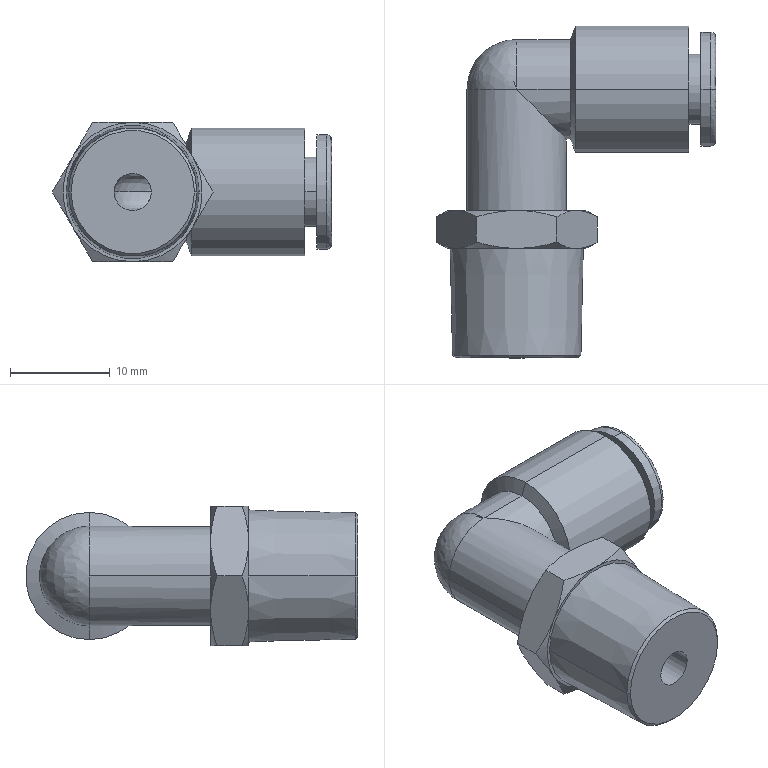Part | SolidWorks | features BaseBody 1 | 1 solid | 52 faces | box 28.083 x 33.4 x 14 mm | volume 4394 mm3 | cone 18 | cylinder 14 | plane 13 | spline 7 | commonest cylinder face diameters 10 x4 3.75 x2 6 x2 7 x2 11.5 x2 12.8 x2